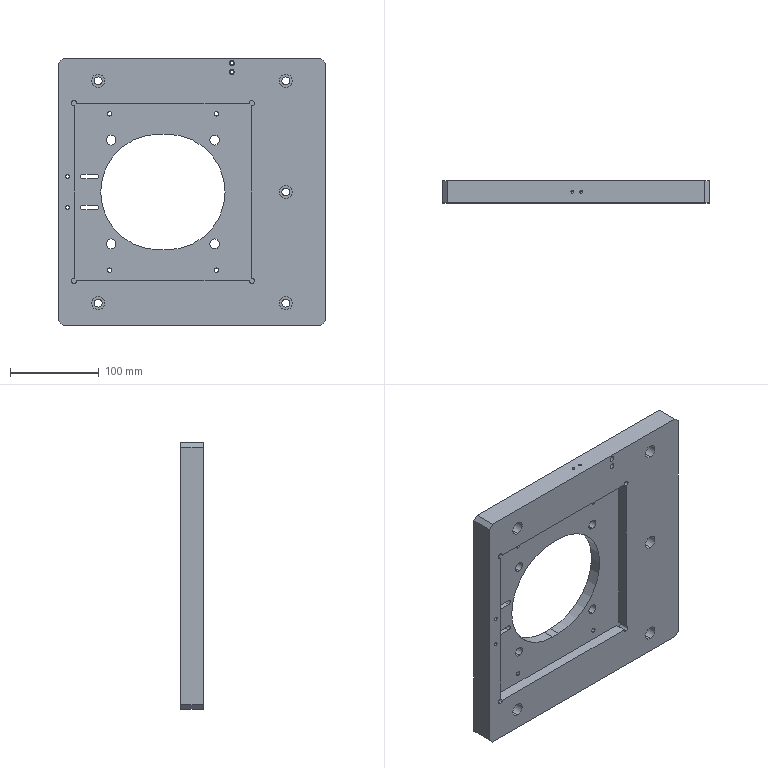Part | SolidWorks | features HoleWzd 9, Cut 2, Chamfer 1, Extrusion 1 | 1 solid | 104 faces | box 300 x 25 x 300 mm | volume 1546097 mm3 | cylinder 68 | plane 28 | cone 8 | commonest cylinder face diameters 6 x10 9 x10 15 x10 5 x8 11 x8 3.3 x4